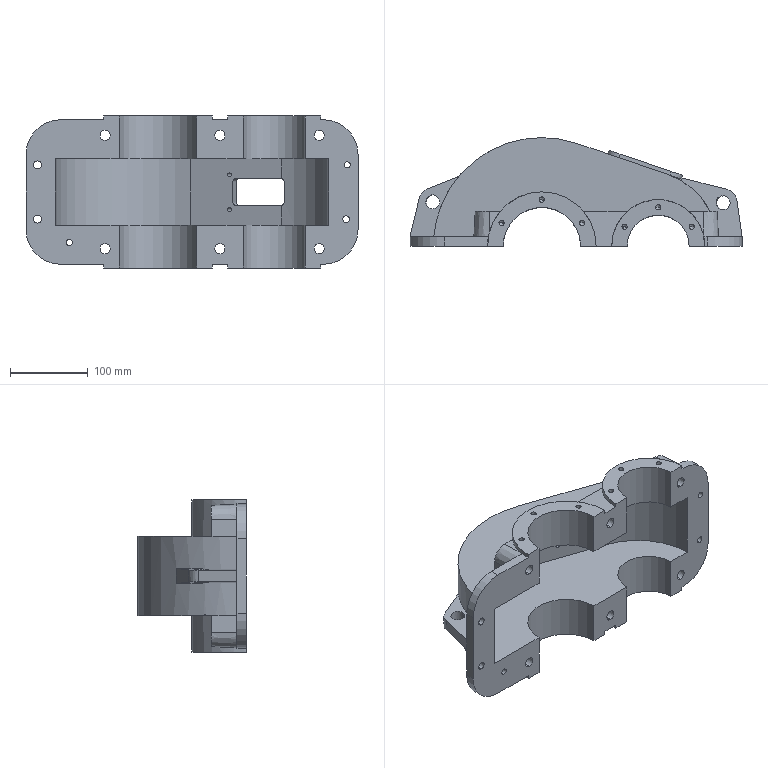Part | SolidWorks | features ICE 21, 3DProfileFeature 10, HoleWzd 10, MirrorPattern 10, Draft 8, Fillet 8, CirPattern 2, Rib 2, Extrusion 1, LPattern 1 | 1 solid | 201 faces | box 428 x 140 x 196 mm | volume 1973144 mm3 | cylinder 102 | plane 71 | cone 28 | commonest cylinder face diameters 6.8 x24 30 x16 13 x12 5 x8 10 x8 18 x5